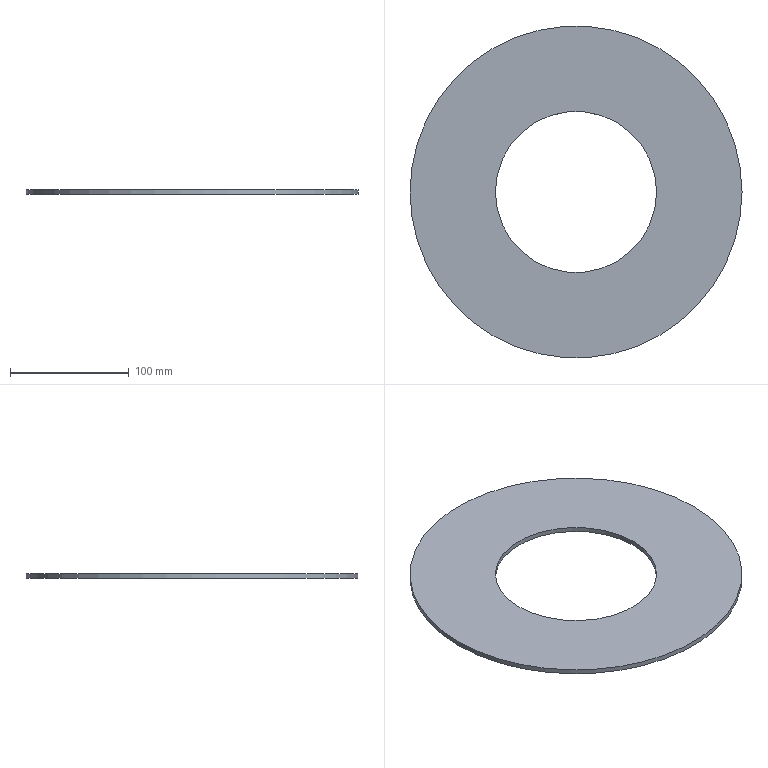Part | NX | features BREP 1, DATUM_CSYS 1 | 1 solid | 4 faces | box 280 x 280 x 4 mm | volume 188194 mm3 | cylinder 2 | plane 2 | commonest cylinder face diameters 136 x1 280 x1
STEP:
#1=CARTESIAN_POINT('',(-140.,0.,20.));
#2=VERTEX_POINT('',#1);
#3=CARTESIAN_POINT('',(0.,0.,20.));
#4=DIRECTION('',(0.,0.,1.));
#5=DIRECTION('',(-1.,0.,0.));
#6=AXIS2_PLACEMENT_3D('',#3,#4,#5);
#7=CIRCLE('',#6,140.);
#8=EDGE_CURVE('',#2,#2,#7,.T.);
#9=ORIENTED_EDGE('',*,*,#8,.F.);
#10=EDGE_LOOP('',(#9));
#11=FACE_BOUND('',#10,.T.);
#12=CARTESIAN_POINT('',(-140.,0.,16.));
#13=VERTEX_POINT('',#12);
#14=CARTESIAN_POINT('',(0.,0.,16.));
#15=DIRECTION('',(0.,0.,1.));
#16=DIRECTION('',(-1.,0.,0.));
#17=AXIS2_PLACEMENT_3D('',#14,#15,#16);
#18=CIRCLE('',#17,140.);
#19=EDGE_CURVE('',#13,#13,#18,.T.);
#20=ORIENTED_EDGE('',*,*,#19,.T.);
#21=EDGE_LOOP('',(#20));
#22=FACE_BOUND('',#21,.T.);
#23=CARTESIAN_POINT('',(0.,0.,20.));
#24=DIRECTION('',(0.,0.,-1.));
#25=DIRECTION('',(-1.,0.,0.));
#26=AXIS2_PLACEMENT_3D('',#23,#24,#25);
#27=CYLINDRICAL_SURFACE('',#26,140.);
#28=ADVANCED_FACE('',(#11,#22),#27,.T.);
#29=CARTESIAN_POINT('',(-68.,0.,20.));
#30=VERTEX_POINT('',#29);
#31=CARTESIAN_POINT('',(0.,0.,20.));
#32=DIRECTION('',(0.,0.,-1.));
#33=DIRECTION('',(-1.,0.,0.));
#34=AXIS2_PLACEMENT_3D('',#31,#32,#33);
#35=CIRCLE('',#34,68.);
#36=EDGE_CURVE('',#30,#30,#35,.T.);
#37=ORIENTED_EDGE('',*,*,#36,.F.);
#38=EDGE_LOOP('',(#37));
#39=FACE_BOUND('',#38,.T.);
#40=CARTESIAN_POINT('',(-68.,0.,16.));
#41=VERTEX_POINT('',#40);
#42=CARTESIAN_POINT('',(0.,0.,16.));
#43=DIRECTION('',(0.,0.,-1.));
#44=DIRECTION('',(-1.,0.,0.));
#45=AXIS2_PLACEMENT_3D('',#42,#43,#44);
#46=CIRCLE('',#45,68.);
#47=EDGE_CURVE('',#41,#41,#46,.T.);
#48=ORIENTED_EDGE('',*,*,#47,.T.);
#49=EDGE_LOOP('',(#48));
#50=FACE_BOUND('',#49,.T.);
#51=CARTESIAN_POINT('',(0.,0.,20.));
#52=DIRECTION('',(0.,0.,-1.));
#53=DIRECTION('',(-1.,0.,0.));
#54=AXIS2_PLACEMENT_3D('',#51,#52,#53);
#55=CYLINDRICAL_SURFACE('',#54,68.);
#56=ADVANCED_FACE('',(#39,#50),#55,.F.);
#57=ORIENTED_EDGE('',*,*,#8,.T.);
#58=EDGE_LOOP('',(#57));
#59=FACE_BOUND('',#58,.T.);
#60=ORIENTED_EDGE('',*,*,#36,.T.);
#61=EDGE_LOOP('',(#60));
#62=FACE_BOUND('',#61,.T.);
#63=CARTESIAN_POINT('',(0.,0.,20.));
#64=DIRECTION('',(0.,0.,1.));
#65=DIRECTION('',(1.,0.,0.));
#66=AXIS2_PLACEMENT_3D('',#63,#64,#65);
#67=PLANE('',#66);
#68=ADVANCED_FACE('',(#59,#62),#67,.T.);
#69=ORIENTED_EDGE('',*,*,#19,.F.);
#70=EDGE_LOOP('',(#69));
#71=FACE_BOUND('',#70,.T.);
#72=ORIENTED_EDGE('',*,*,#47,.F.);
#73=EDGE_LOOP('',(#72));
#74=FACE_BOUND('',#73,.T.);
#75=CARTESIAN_POINT('',(0.,0.,16.));
#76=DIRECTION('',(0.,0.,1.));
#77=DIRECTION('',(1.,0.,0.));
#78=AXIS2_PLACEMENT_3D('',#75,#76,#77);
#79=PLANE('',#78);
#80=ADVANCED_FACE('',(#71,#74),#79,.F.);
#81=CLOSED_SHELL('',(#28,#56,#68,#80));
#82=MANIFOLD_SOLID_BREP('',#81);
#83=(LENGTH_UNIT()NAMED_UNIT(*)SI_UNIT(.MILLI.,.METRE.));
#84=UNCERTAINTY_MEASURE_WITH_UNIT(LENGTH_MEASURE(0.00001),#83,'','');
#85=(NAMED_UNIT(*)PLANE_ANGLE_UNIT()SI_UNIT($,.RADIAN.));
#86=(NAMED_UNIT(*)SI_UNIT($,.STERADIAN.)SOLID_ANGLE_UNIT());
#87=(GEOMETRIC_REPRESENTATION_CONTEXT(3)GLOBAL_UNCERTAINTY_ASSIGNED_CONTEXT((#84))GLOBAL_UNIT_ASSIGNED_CONTEXT((#83,#85,#86))REPRESENTATION_CONTEXT('',''));
#88=ADVANCED_BREP_SHAPE_REPRESENTATION('',(#82),#87);